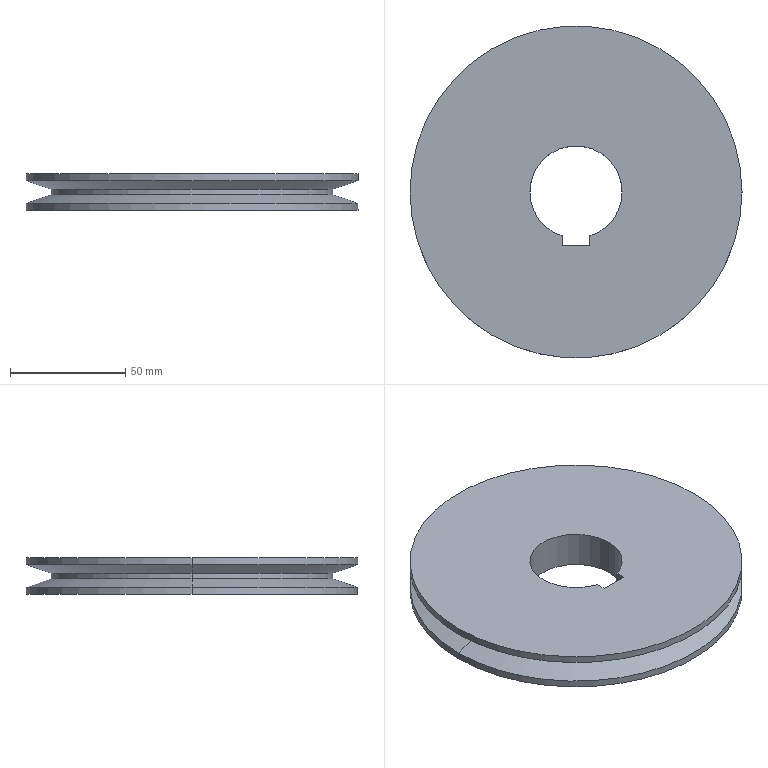Part | SolidWorks | features ICE 2, BaseBody 1 | 1 solid | 18 faces | box 144 x 144 x 16 mm | volume 211309 mm3 | cylinder 9 | plane 5 | cone 4 | commonest cylinder face diameters 144 x4 40 x3 122 x2
STEP:
#1=CARTESIAN_POINT('',(-20.,0.,0.));
#2=VERTEX_POINT('',#1);
#3=CARTESIAN_POINT('',(-6.,-19.079,0.));
#4=VERTEX_POINT('',#3);
#5=CARTESIAN_POINT('',(0.,0.,0.));
#6=DIRECTION('',(0.,0.,1.));
#7=DIRECTION('',(1.,0.,0.));
#8=AXIS2_PLACEMENT_3D('',#5,#6,#7);
#9=CIRCLE('',#8,20.);
#10=EDGE_CURVE('',#2,#4,#9,.T.);
#11=ORIENTED_EDGE('',*,*,#10,.F.);
#12=CARTESIAN_POINT('',(-20.,0.,16.));
#13=VERTEX_POINT('',#12);
#14=CARTESIAN_POINT('',(-20.,0.,0.));
#15=DIRECTION('',(0.,0.,1.));
#16=VECTOR('',#15,1000.);
#17=LINE('',#14,#16);
#18=EDGE_CURVE('',#2,#13,#17,.T.);
#19=ORIENTED_EDGE('',*,*,#18,.T.);
#20=CARTESIAN_POINT('',(-6.,-19.079,16.));
#21=VERTEX_POINT('',#20);
#22=CARTESIAN_POINT('',(0.,0.,16.));
#23=DIRECTION('',(0.,0.,1.));
#24=DIRECTION('',(1.,0.,0.));
#25=AXIS2_PLACEMENT_3D('',#22,#23,#24);
#26=CIRCLE('',#25,20.);
#27=EDGE_CURVE('',#13,#21,#26,.T.);
#28=ORIENTED_EDGE('',*,*,#27,.T.);
#29=CARTESIAN_POINT('',(-6.,-19.079,0.));
#30=DIRECTION('',(0.,0.,-1.));
#31=VECTOR('',#30,1000.);
#32=LINE('',#29,#31);
#33=EDGE_CURVE('',#21,#4,#32,.T.);
#34=ORIENTED_EDGE('',*,*,#33,.T.);
#35=EDGE_LOOP('',(#11,#19,#28,#34));
#36=FACE_OUTER_BOUND('',#35,.T.);
#37=CARTESIAN_POINT('',(0.,0.,0.));
#38=DIRECTION('',(0.,0.,1.));
#39=DIRECTION('',(1.,0.,0.));
#40=AXIS2_PLACEMENT_3D('',#37,#38,#39);
#41=CYLINDRICAL_SURFACE('',#40,20.);
#42=ADVANCED_FACE('',(#36),#41,.F.);
#43=ORIENTED_EDGE('',*,*,#18,.F.);
#44=CARTESIAN_POINT('',(20.,0.,0.));
#45=VERTEX_POINT('',#44);
#46=CARTESIAN_POINT('',(0.,0.,0.));
#47=DIRECTION('',(0.,0.,1.));
#48=DIRECTION('',(1.,0.,0.));
#49=AXIS2_PLACEMENT_3D('',#46,#47,#48);
#50=CIRCLE('',#49,20.);
#51=EDGE_CURVE('',#45,#2,#50,.T.);
#52=ORIENTED_EDGE('',*,*,#51,.F.);
#53=CARTESIAN_POINT('',(20.,0.,16.));
#54=VERTEX_POINT('',#53);
#55=CARTESIAN_POINT('',(20.,0.,0.));
#56=DIRECTION('',(0.,0.,1.));
#57=VECTOR('',#56,1000.);
#58=LINE('',#55,#57);
#59=EDGE_CURVE('',#45,#54,#58,.T.);
#60=ORIENTED_EDGE('',*,*,#59,.T.);
#61=CARTESIAN_POINT('',(0.,0.,16.));
#62=DIRECTION('',(0.,0.,1.));
#63=DIRECTION('',(1.,0.,0.));
#64=AXIS2_PLACEMENT_3D('',#61,#62,#63);
#65=CIRCLE('',#64,20.);
#66=EDGE_CURVE('',#54,#13,#65,.T.);
#67=ORIENTED_EDGE('',*,*,#66,.T.);
#68=EDGE_LOOP('',(#43,#52,#60,#67));
#69=FACE_OUTER_BOUND('',#68,.T.);
#70=CARTESIAN_POINT('',(0.,0.,0.));
#71=DIRECTION('',(0.,0.,1.));
#72=DIRECTION('',(1.,0.,0.));
#73=AXIS2_PLACEMENT_3D('',#70,#71,#72);
#74=CYLINDRICAL_SURFACE('',#73,20.);
#75=ADVANCED_FACE('',(#69),#74,.F.);
#76=CARTESIAN_POINT('',(-72.,0.,3.061));
#77=VERTEX_POINT('',#76);
#78=CARTESIAN_POINT('',(72.,0.,3.061));
#79=VERTEX_POINT('',#78);
#80=CARTESIAN_POINT('',(0.,0.,3.061));
#81=DIRECTION('',(0.,0.,-1.));
#82=DIRECTION('',(-1.,0.,0.));
#83=AXIS2_PLACEMENT_3D('',#80,#81,#82);
#84=CIRCLE('',#83,72.);
#85=EDGE_CURVE('',#77,#79,#84,.T.);
#86=ORIENTED_EDGE('',*,*,#85,.T.);
#87=CARTESIAN_POINT('',(72.,0.,0.));
#88=VERTEX_POINT('',#87);
#89=CARTESIAN_POINT('',(72.,0.,8.));
#90=DIRECTION('',(0.,0.,-1.));
#91=VECTOR('',#90,1000.);
#92=LINE('',#89,#91);
#93=EDGE_CURVE('',#79,#88,#92,.T.);
#94=ORIENTED_EDGE('',*,*,#93,.T.);
#95=CARTESIAN_POINT('',(-72.,0.,0.));
#96=VERTEX_POINT('',#95);
#97=CARTESIAN_POINT('',(0.,0.,0.));
#98=DIRECTION('',(0.,0.,-1.));
#99=DIRECTION('',(-1.,0.,0.));
#100=AXIS2_PLACEMENT_3D('',#97,#98,#99);
#101=CIRCLE('',#100,72.);
#102=EDGE_CURVE('',#96,#88,#101,.T.);
#103=ORIENTED_EDGE('',*,*,#102,.F.);
#104=CARTESIAN_POINT('',(-72.,0.,8.));
#105=DIRECTION('',(0.,0.,-1.));
#106=VECTOR('',#105,1000.);
#107=LINE('',#104,#106);
#108=EDGE_CURVE('',#77,#96,#107,.T.);
#109=ORIENTED_EDGE('',*,*,#108,.F.);
#110=EDGE_LOOP('',(#86,#94,#103,#109));
#111=FACE_OUTER_BOUND('',#110,.T.);
#112=CARTESIAN_POINT('',(0.,0.,8.));
#113=DIRECTION('',(0.,0.,-1.));
#114=DIRECTION('',(-1.,0.,0.));
#115=AXIS2_PLACEMENT_3D('',#112,#113,#114);
#116=CYLINDRICAL_SURFACE('',#115,72.);
#117=ADVANCED_FACE('',(#111),#116,.T.);
#118=CARTESIAN_POINT('',(-61.,0.,6.849));
#119=VERTEX_POINT('',#118);
#120=CARTESIAN_POINT('',(61.,0.,6.849));
#121=VERTEX_POINT('',#120);
#122=CARTESIAN_POINT('',(0.,0.,6.849));
#123=DIRECTION('',(0.,0.,-1.));
#124=DIRECTION('',(0.,1.,0.));
#125=AXIS2_PLACEMENT_3D('',#122,#123,#124);
#126=CIRCLE('',#125,61.);
#127=EDGE_CURVE('',#119,#121,#126,.T.);
#128=ORIENTED_EDGE('',*,*,#127,.T.);
#129=CARTESIAN_POINT('',(72.,0.,3.061));
#130=DIRECTION('',(0.9455,0.,-0.3256));
#131=VECTOR('',#130,1000.);
#132=LINE('',#129,#131);
#133=EDGE_CURVE('',#121,#79,#132,.T.);
#134=ORIENTED_EDGE('',*,*,#133,.T.);
#135=ORIENTED_EDGE('',*,*,#85,.F.);
#136=CARTESIAN_POINT('',(-72.,0.,3.061));
#137=DIRECTION('',(-0.9455,0.,-0.3256));
#138=VECTOR('',#137,1000.);
#139=LINE('',#136,#138);
#140=EDGE_CURVE('',#119,#77,#139,.T.);
#141=ORIENTED_EDGE('',*,*,#140,.F.);
#142=EDGE_LOOP('',(#128,#134,#135,#141));
#143=FACE_OUTER_BOUND('',#142,.T.);
#144=CARTESIAN_POINT('',(0.,0.,3.061));
#145=DIRECTION('',(0.,0.,-1.));
#146=DIRECTION('',(-1.,0.,0.));
#147=AXIS2_PLACEMENT_3D('',#144,#145,#146);
#148=CONICAL_SURFACE('',#147,72.,1.239);
#149=ADVANCED_FACE('',(#143),#148,.T.);
#150=ORIENTED_EDGE('',*,*,#127,.F.);
#151=CARTESIAN_POINT('',(-61.,0.,9.151));
#152=VERTEX_POINT('',#151);
#153=CARTESIAN_POINT('',(-61.,0.,8.));
#154=DIRECTION('',(0.,0.,1.));
#155=VECTOR('',#154,1000.);
#156=LINE('',#153,#155);
#157=EDGE_CURVE('',#119,#152,#156,.T.);
#158=ORIENTED_EDGE('',*,*,#157,.T.);
#159=CARTESIAN_POINT('',(61.,0.,9.151));
#160=VERTEX_POINT('',#159);
#161=CARTESIAN_POINT('',(0.,0.,9.151));
#162=DIRECTION('',(0.,0.,-1.));
#163=DIRECTION('',(1.,0.,0.));
#164=AXIS2_PLACEMENT_3D('',#161,#162,#163);
#165=CIRCLE('',#164,61.);
#166=EDGE_CURVE('',#152,#160,#165,.T.);
#167=ORIENTED_EDGE('',*,*,#166,.T.);
#168=CARTESIAN_POINT('',(61.,0.,8.));
#169=DIRECTION('',(0.,0.,1.));
#170=VECTOR('',#169,1000.);
#171=LINE('',#168,#170);
#172=EDGE_CURVE('',#121,#160,#171,.T.);
#173=ORIENTED_EDGE('',*,*,#172,.F.);
#174=EDGE_LOOP('',(#150,#158,#167,#173));
#175=FACE_OUTER_BOUND('',#174,.T.);
#176=CARTESIAN_POINT('',(0.,0.,8.));
#177=DIRECTION('',(0.,0.,1.));
#178=DIRECTION('',(1.,0.,0.));
#179=AXIS2_PLACEMENT_3D('',#176,#177,#178);
#180=CYLINDRICAL_SURFACE('',#179,61.);
#181=ADVANCED_FACE('',(#175),#180,.T.);
#182=ORIENTED_EDGE('',*,*,#166,.F.);
#183=CARTESIAN_POINT('',(-72.,0.,12.939));
#184=VERTEX_POINT('',#183);
#185=CARTESIAN_POINT('',(-72.,0.,12.939));
#186=DIRECTION('',(-0.9455,0.,0.3256));
#187=VECTOR('',#186,1000.);
#188=LINE('',#185,#187);
#189=EDGE_CURVE('',#152,#184,#188,.T.);
#190=ORIENTED_EDGE('',*,*,#189,.T.);
#191=CARTESIAN_POINT('',(72.,0.,12.939));
#192=VERTEX_POINT('',#191);
#193=CARTESIAN_POINT('',(0.,0.,12.939));
#194=DIRECTION('',(0.,0.,-1.));
#195=DIRECTION('',(0.,1.,0.));
#196=AXIS2_PLACEMENT_3D('',#193,#194,#195);
#197=CIRCLE('',#196,72.);
#198=EDGE_CURVE('',#184,#192,#197,.T.);
#199=ORIENTED_EDGE('',*,*,#198,.T.);
#200=CARTESIAN_POINT('',(72.,0.,12.939));
#201=DIRECTION('',(0.9455,0.,0.3256));
#202=VECTOR('',#201,1000.);
#203=LINE('',#200,#202);
#204=EDGE_CURVE('',#160,#192,#203,.T.);
#205=ORIENTED_EDGE('',*,*,#204,.F.);
#206=EDGE_LOOP('',(#182,#190,#199,#205));
#207=FACE_OUTER_BOUND('',#206,.T.);
#208=CARTESIAN_POINT('',(0.,0.,12.939));
#209=DIRECTION('',(0.,0.,1.));
#210=DIRECTION('',(1.,0.,0.));
#211=AXIS2_PLACEMENT_3D('',#208,#209,#210);
#212=CONICAL_SURFACE('',#211,72.,1.239);
#213=ADVANCED_FACE('',(#207),#212,.T.);
#214=CARTESIAN_POINT('',(-72.,0.,16.));
#215=VERTEX_POINT('',#214);
#216=CARTESIAN_POINT('',(72.,0.,16.));
#217=VERTEX_POINT('',#216);
#218=CARTESIAN_POINT('',(0.,0.,16.));
#219=DIRECTION('',(0.,0.,-1.));
#220=DIRECTION('',(-1.,0.,0.));
#221=AXIS2_PLACEMENT_3D('',#218,#219,#220);
#222=CIRCLE('',#221,72.);
#223=EDGE_CURVE('',#215,#217,#222,.T.);
#224=ORIENTED_EDGE('',*,*,#223,.T.);
#225=CARTESIAN_POINT('',(72.,0.,8.));
#226=DIRECTION('',(0.,0.,-1.));
#227=VECTOR('',#226,1000.);
#228=LINE('',#225,#227);
#229=EDGE_CURVE('',#217,#192,#228,.T.);
#230=ORIENTED_EDGE('',*,*,#229,.T.);
#231=ORIENTED_EDGE('',*,*,#198,.F.);
#232=CARTESIAN_POINT('',(-72.,0.,8.));
#233=DIRECTION('',(0.,0.,-1.));
#234=VECTOR('',#233,1000.);
#235=LINE('',#232,#234);
#236=EDGE_CURVE('',#215,#184,#235,.T.);
#237=ORIENTED_EDGE('',*,*,#236,.F.);
#238=EDGE_LOOP('',(#224,#230,#231,#237));
#239=FACE_OUTER_BOUND('',#238,.T.);
#240=CARTESIAN_POINT('',(0.,0.,8.));
#241=DIRECTION('',(0.,0.,-1.));
#242=DIRECTION('',(-1.,0.,0.));
#243=AXIS2_PLACEMENT_3D('',#240,#241,#242);
#244=CYLINDRICAL_SURFACE('',#243,72.);
#245=ADVANCED_FACE('',(#239),#244,.T.);
#246=CARTESIAN_POINT('',(-6.,-23.3,0.));
#247=VERTEX_POINT('',#246);
#248=CARTESIAN_POINT('',(-6.,0.,0.));
#249=DIRECTION('',(0.,-1.,0.));
#250=VECTOR('',#249,1000.);
#251=LINE('',#248,#250);
#252=EDGE_CURVE('',#4,#247,#251,.T.);
#253=ORIENTED_EDGE('',*,*,#252,.T.);
#254=CARTESIAN_POINT('',(6.,-23.3,0.));
#255=VERTEX_POINT('',#254);
#256=CARTESIAN_POINT('',(-6.,-23.3,0.));
#257=DIRECTION('',(1.,0.,0.));
#258=VECTOR('',#257,1000.);
#259=LINE('',#256,#258);
#260=EDGE_CURVE('',#247,#255,#259,.T.);
#261=ORIENTED_EDGE('',*,*,#260,.T.);
#262=CARTESIAN_POINT('',(6.,-19.079,0.));
#263=VERTEX_POINT('',#262);
#264=CARTESIAN_POINT('',(6.,0.,0.));
#265=DIRECTION('',(0.,1.,0.));
#266=VECTOR('',#265,1000.);
#267=LINE('',#264,#266);
#268=EDGE_CURVE('',#255,#263,#267,.T.);
#269=ORIENTED_EDGE('',*,*,#268,.T.);
#270=CARTESIAN_POINT('',(0.,0.,0.));
#271=DIRECTION('',(0.,0.,1.));
#272=DIRECTION('',(1.,0.,0.));
#273=AXIS2_PLACEMENT_3D('',#270,#271,#272);
#274=CIRCLE('',#273,20.);
#275=EDGE_CURVE('',#263,#45,#274,.T.);
#276=ORIENTED_EDGE('',*,*,#275,.T.);
#277=ORIENTED_EDGE('',*,*,#51,.T.);
#278=ORIENTED_EDGE('',*,*,#10,.T.);
#279=EDGE_LOOP('',(#253,#261,#269,#276,#277,#278));
#280=FACE_BOUND('',#279,.T.);
#281=ORIENTED_EDGE('',*,*,#102,.T.);
#282=CARTESIAN_POINT('',(0.,0.,0.));
#283=DIRECTION('',(0.,0.,-1.));
#284=DIRECTION('',(-1.,0.,0.));
#285=AXIS2_PLACEMENT_3D('',#282,#283,#284);
#286=CIRCLE('',#285,72.);
#287=EDGE_CURVE('',#88,#96,#286,.T.);
#288=ORIENTED_EDGE('',*,*,#287,.T.);
#289=EDGE_LOOP('',(#281,#288));
#290=FACE_OUTER_BOUND('',#289,.T.);
#291=CARTESIAN_POINT('',(0.,36.,0.));
#292=DIRECTION('',(0.,0.,-1.));
#293=DIRECTION('',(-1.,0.,0.));
#294=AXIS2_PLACEMENT_3D('',#291,#292,#293);
#295=PLANE('',#294);
#296=ADVANCED_FACE('',(#280,#290),#295,.T.);
#297=ORIENTED_EDGE('',*,*,#93,.F.);
#298=CARTESIAN_POINT('',(0.,0.,3.061));
#299=DIRECTION('',(0.,0.,-1.));
#300=DIRECTION('',(-1.,0.,0.));
#301=AXIS2_PLACEMENT_3D('',#298,#299,#300);
#302=CIRCLE('',#301,72.);
#303=EDGE_CURVE('',#79,#77,#302,.T.);
#304=ORIENTED_EDGE('',*,*,#303,.T.);
#305=ORIENTED_EDGE('',*,*,#108,.T.);
#306=ORIENTED_EDGE('',*,*,#287,.F.);
#307=EDGE_LOOP('',(#297,#304,#305,#306));
#308=FACE_OUTER_BOUND('',#307,.T.);
#309=CARTESIAN_POINT('',(0.,0.,8.));
#310=DIRECTION('',(0.,0.,-1.));
#311=DIRECTION('',(-1.,0.,0.));
#312=AXIS2_PLACEMENT_3D('',#309,#310,#311);
#313=CYLINDRICAL_SURFACE('',#312,72.);
#314=ADVANCED_FACE('',(#308),#313,.T.);
#315=ORIENTED_EDGE('',*,*,#133,.F.);
#316=CARTESIAN_POINT('',(0.,0.,6.849));
#317=DIRECTION('',(0.,0.,-1.));
#318=DIRECTION('',(0.,1.,0.));
#319=AXIS2_PLACEMENT_3D('',#316,#317,#318);
#320=CIRCLE('',#319,61.);
#321=EDGE_CURVE('',#121,#119,#320,.T.);
#322=ORIENTED_EDGE('',*,*,#321,.T.);
#323=ORIENTED_EDGE('',*,*,#140,.T.);
#324=ORIENTED_EDGE('',*,*,#303,.F.);
#325=EDGE_LOOP('',(#315,#322,#323,#324));
#326=FACE_OUTER_BOUND('',#325,.T.);
#327=CARTESIAN_POINT('',(0.,0.,3.061));
#328=DIRECTION('',(0.,0.,-1.));
#329=DIRECTION('',(-1.,0.,0.));
#330=AXIS2_PLACEMENT_3D('',#327,#328,#329);
#331=CONICAL_SURFACE('',#330,72.,1.239);
#332=ADVANCED_FACE('',(#326),#331,.T.);
#333=ORIENTED_EDGE('',*,*,#157,.F.);
#334=ORIENTED_EDGE('',*,*,#321,.F.);
#335=ORIENTED_EDGE('',*,*,#172,.T.);
#336=CARTESIAN_POINT('',(0.,0.,9.151));
#337=DIRECTION('',(0.,0.,-1.));
#338=DIRECTION('',(1.,0.,0.));
#339=AXIS2_PLACEMENT_3D('',#336,#337,#338);
#340=CIRCLE('',#339,61.);
#341=EDGE_CURVE('',#160,#152,#340,.T.);
#342=ORIENTED_EDGE('',*,*,#341,.T.);
#343=EDGE_LOOP('',(#333,#334,#335,#342));
#344=FACE_OUTER_BOUND('',#343,.T.);
#345=CARTESIAN_POINT('',(0.,0.,8.));
#346=DIRECTION('',(0.,0.,1.));
#347=DIRECTION('',(1.,0.,0.));
#348=AXIS2_PLACEMENT_3D('',#345,#346,#347);
#349=CYLINDRICAL_SURFACE('',#348,61.);
#350=ADVANCED_FACE('',(#344),#349,.T.);
#351=ORIENTED_EDGE('',*,*,#189,.F.);
#352=ORIENTED_EDGE('',*,*,#341,.F.);
#353=ORIENTED_EDGE('',*,*,#204,.T.);
#354=CARTESIAN_POINT('',(0.,0.,12.939));
#355=DIRECTION('',(0.,0.,-1.));
#356=DIRECTION('',(0.,1.,0.));
#357=AXIS2_PLACEMENT_3D('',#354,#355,#356);
#358=CIRCLE('',#357,72.);
#359=EDGE_CURVE('',#192,#184,#358,.T.);
#360=ORIENTED_EDGE('',*,*,#359,.T.);
#361=EDGE_LOOP('',(#351,#352,#353,#360));
#362=FACE_OUTER_BOUND('',#361,.T.);
#363=CARTESIAN_POINT('',(0.,0.,12.939));
#364=DIRECTION('',(0.,0.,1.));
#365=DIRECTION('',(1.,0.,0.));
#366=AXIS2_PLACEMENT_3D('',#363,#364,#365);
#367=CONICAL_SURFACE('',#366,72.,1.239);
#368=ADVANCED_FACE('',(#362),#367,.T.);
#369=ORIENTED_EDGE('',*,*,#229,.F.);
#370=CARTESIAN_POINT('',(0.,0.,16.));
#371=DIRECTION('',(0.,0.,-1.));
#372=DIRECTION('',(-1.,0.,0.));
#373=AXIS2_PLACEMENT_3D('',#370,#371,#372);
#374=CIRCLE('',#373,72.);
#375=EDGE_CURVE('',#217,#215,#374,.T.);
#376=ORIENTED_EDGE('',*,*,#375,.T.);
#377=ORIENTED_EDGE('',*,*,#236,.T.);
#378=ORIENTED_EDGE('',*,*,#359,.F.);
#379=EDGE_LOOP('',(#369,#376,#377,#378));
#380=FACE_OUTER_BOUND('',#379,.T.);
#381=CARTESIAN_POINT('',(0.,0.,8.));
#382=DIRECTION('',(0.,0.,-1.));
#383=DIRECTION('',(-1.,0.,0.));
#384=AXIS2_PLACEMENT_3D('',#381,#382,#383);
#385=CYLINDRICAL_SURFACE('',#384,72.);
#386=ADVANCED_FACE('',(#380),#385,.T.);
#387=CARTESIAN_POINT('',(-6.,-23.3,16.));
#388=VERTEX_POINT('',#387);
#389=CARTESIAN_POINT('',(-6.,0.,16.));
#390=DIRECTION('',(0.,-1.,0.));
#391=VECTOR('',#390,1000.);
#392=LINE('',#389,#391);
#393=EDGE_CURVE('',#21,#388,#392,.T.);
#394=ORIENTED_EDGE('',*,*,#393,.F.);
#395=ORIENTED_EDGE('',*,*,#27,.F.);
#396=ORIENTED_EDGE('',*,*,#66,.F.);
#397=CARTESIAN_POINT('',(6.,-19.079,16.));
#398=VERTEX_POINT('',#397);
#399=CARTESIAN_POINT('',(0.,0.,16.));
#400=DIRECTION('',(0.,0.,1.));
#401=DIRECTION('',(1.,0.,0.));
#402=AXIS2_PLACEMENT_3D('',#399,#400,#401);
#403=CIRCLE('',#402,20.);
#404=EDGE_CURVE('',#398,#54,#403,.T.);
#405=ORIENTED_EDGE('',*,*,#404,.F.);
#406=CARTESIAN_POINT('',(6.,-23.3,16.));
#407=VERTEX_POINT('',#406);
#408=CARTESIAN_POINT('',(6.,0.,16.));
#409=DIRECTION('',(0.,1.,0.));
#410=VECTOR('',#409,1000.);
#411=LINE('',#408,#410);
#412=EDGE_CURVE('',#407,#398,#411,.T.);
#413=ORIENTED_EDGE('',*,*,#412,.F.);
#414=CARTESIAN_POINT('',(-6.,-23.3,16.));
#415=DIRECTION('',(1.,0.,0.));
#416=VECTOR('',#415,1000.);
#417=LINE('',#414,#416);
#418=EDGE_CURVE('',#388,#407,#417,.T.);
#419=ORIENTED_EDGE('',*,*,#418,.F.);
#420=EDGE_LOOP('',(#394,#395,#396,#405,#413,#419));
#421=FACE_BOUND('',#420,.T.);
#422=ORIENTED_EDGE('',*,*,#223,.F.);
#423=ORIENTED_EDGE('',*,*,#375,.F.);
#424=EDGE_LOOP('',(#422,#423));
#425=FACE_OUTER_BOUND('',#424,.T.);
#426=CARTESIAN_POINT('',(0.,36.,16.));
#427=DIRECTION('',(0.,0.,1.));
#428=DIRECTION('',(1.,0.,0.));
#429=AXIS2_PLACEMENT_3D('',#426,#427,#428);
#430=PLANE('',#429);
#431=ADVANCED_FACE('',(#421,#425),#430,.T.);
#432=ORIENTED_EDGE('',*,*,#59,.F.);
#433=ORIENTED_EDGE('',*,*,#275,.F.);
#434=CARTESIAN_POINT('',(6.,-19.079,0.));
#435=DIRECTION('',(0.,0.,1.));
#436=VECTOR('',#435,1000.);
#437=LINE('',#434,#436);
#438=EDGE_CURVE('',#263,#398,#437,.T.);
#439=ORIENTED_EDGE('',*,*,#438,.T.);
#440=ORIENTED_EDGE('',*,*,#404,.T.);
#441=EDGE_LOOP('',(#432,#433,#439,#440));
#442=FACE_OUTER_BOUND('',#441,.T.);
#443=CARTESIAN_POINT('',(0.,0.,0.));
#444=DIRECTION('',(0.,0.,1.));
#445=DIRECTION('',(1.,0.,0.));
#446=AXIS2_PLACEMENT_3D('',#443,#444,#445);
#447=CYLINDRICAL_SURFACE('',#446,20.);
#448=ADVANCED_FACE('',(#442),#447,.F.);
#449=ORIENTED_EDGE('',*,*,#393,.T.);
#450=CARTESIAN_POINT('',(-6.,-23.3,0.));
#451=DIRECTION('',(0.,0.,1.));
#452=VECTOR('',#451,1000.);
#453=LINE('',#450,#452);
#454=EDGE_CURVE('',#247,#388,#453,.T.);
#455=ORIENTED_EDGE('',*,*,#454,.F.);
#456=ORIENTED_EDGE('',*,*,#252,.F.);
#457=ORIENTED_EDGE('',*,*,#33,.F.);
#458=EDGE_LOOP('',(#449,#455,#456,#457));
#459=FACE_OUTER_BOUND('',#458,.T.);
#460=CARTESIAN_POINT('',(-6.,0.,0.));
#461=DIRECTION('',(-1.,0.,0.));
#462=DIRECTION('',(0.,-1.,0.));
#463=AXIS2_PLACEMENT_3D('',#460,#461,#462);
#464=PLANE('',#463);
#465=ADVANCED_FACE('',(#459),#464,.F.);
#466=ORIENTED_EDGE('',*,*,#268,.F.);
#467=CARTESIAN_POINT('',(6.,-23.3,0.));
#468=DIRECTION('',(0.,0.,1.));
#469=VECTOR('',#468,1000.);
#470=LINE('',#467,#469);
#471=EDGE_CURVE('',#255,#407,#470,.T.);
#472=ORIENTED_EDGE('',*,*,#471,.T.);
#473=ORIENTED_EDGE('',*,*,#412,.T.);
#474=ORIENTED_EDGE('',*,*,#438,.F.);
#475=EDGE_LOOP('',(#466,#472,#473,#474));
#476=FACE_OUTER_BOUND('',#475,.T.);
#477=CARTESIAN_POINT('',(6.,0.,0.));
#478=DIRECTION('',(1.,0.,0.));
#479=DIRECTION('',(0.,1.,0.));
#480=AXIS2_PLACEMENT_3D('',#477,#478,#479);
#481=PLANE('',#480);
#482=ADVANCED_FACE('',(#476),#481,.F.);
#483=ORIENTED_EDGE('',*,*,#418,.T.);
#484=ORIENTED_EDGE('',*,*,#471,.F.);
#485=ORIENTED_EDGE('',*,*,#260,.F.);
#486=ORIENTED_EDGE('',*,*,#454,.T.);
#487=EDGE_LOOP('',(#483,#484,#485,#486));
#488=FACE_OUTER_BOUND('',#487,.T.);
#489=CARTESIAN_POINT('',(-6.,-23.3,0.));
#490=DIRECTION('',(0.,-1.,0.));
#491=DIRECTION('',(0.,0.,-1.));
#492=AXIS2_PLACEMENT_3D('',#489,#490,#491);
#493=PLANE('',#492);
#494=ADVANCED_FACE('',(#488),#493,.F.);
#495=CLOSED_SHELL('',(#42,#75,#117,#149,#181,#213,#245,#296,#314,#332,#350,#368,#386,#431,#448,#465,#482,#494));
#496=MANIFOLD_SOLID_BREP('',#495);
#497=CARTESIAN_POINT('',(0.,0.,0.));
#498=DIRECTION('',(0.,0.,1.));
#499=DIRECTION('',(1.,0.,0.));
#500=AXIS2_PLACEMENT_3D('',#497,#498,#499);
#501=(LENGTH_UNIT()NAMED_UNIT(*)SI_UNIT(.MILLI.,.METRE.));
#502=UNCERTAINTY_MEASURE_WITH_UNIT(LENGTH_MEASURE(0.00001),#501,'','');
#503=(NAMED_UNIT(*)PLANE_ANGLE_UNIT()SI_UNIT($,.RADIAN.));
#504=(NAMED_UNIT(*)SI_UNIT($,.STERADIAN.)SOLID_ANGLE_UNIT());
#505=(GEOMETRIC_REPRESENTATION_CONTEXT(3)GLOBAL_UNCERTAINTY_ASSIGNED_CONTEXT((#502))GLOBAL_UNIT_ASSIGNED_CONTEXT((#501,#503,#504))REPRESENTATION_CONTEXT('',''));
#506=ADVANCED_BREP_SHAPE_REPRESENTATION('',(#496,#500),#505);